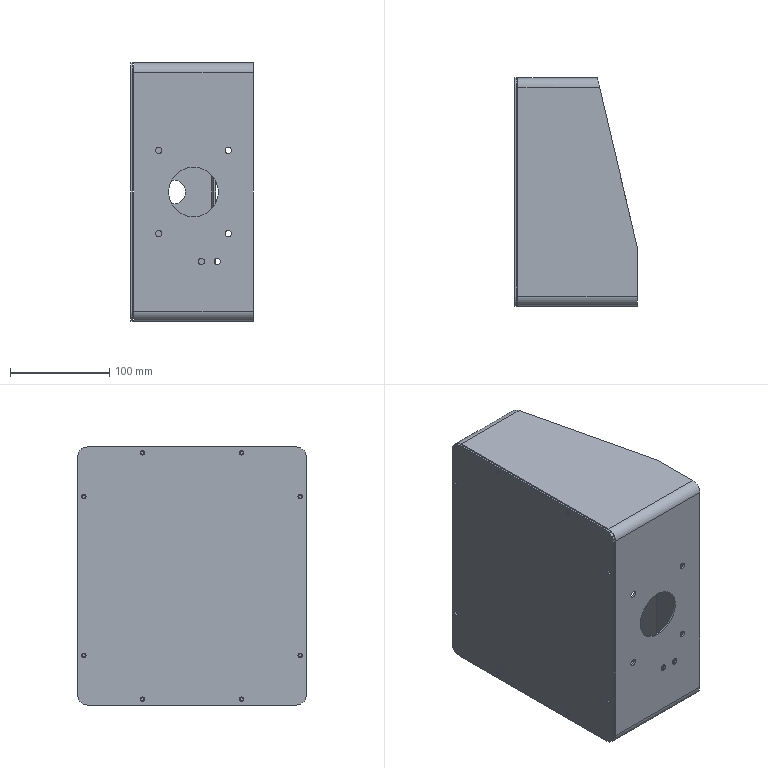Part | STEP file | QA-TE04 | 2 solids | 104 faces | box 123 x 230 x 260 mm | volume 391275 mm3 | cylinder 76 | plane 28 | commonest cylinder face diameters 3.3 x16 4.5 x16 16 x14 6.5 x12 20 x8 4.2 x6